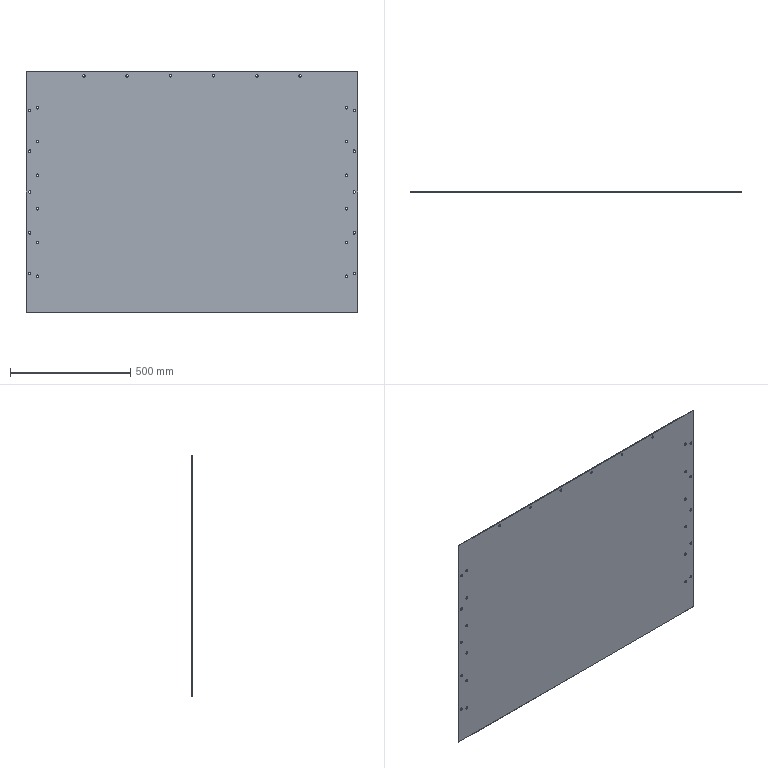Part | SolidWorks | features ICE 2, SMBaseFlange 2, FlatPattern 1, SheetMetal 1 | 1 solid | 62 faces | box 1380 x 3 x 1000 mm | volume 4133403 mm3 | cylinder 56 | plane 6 | commonest cylinder face diameters 10 x56